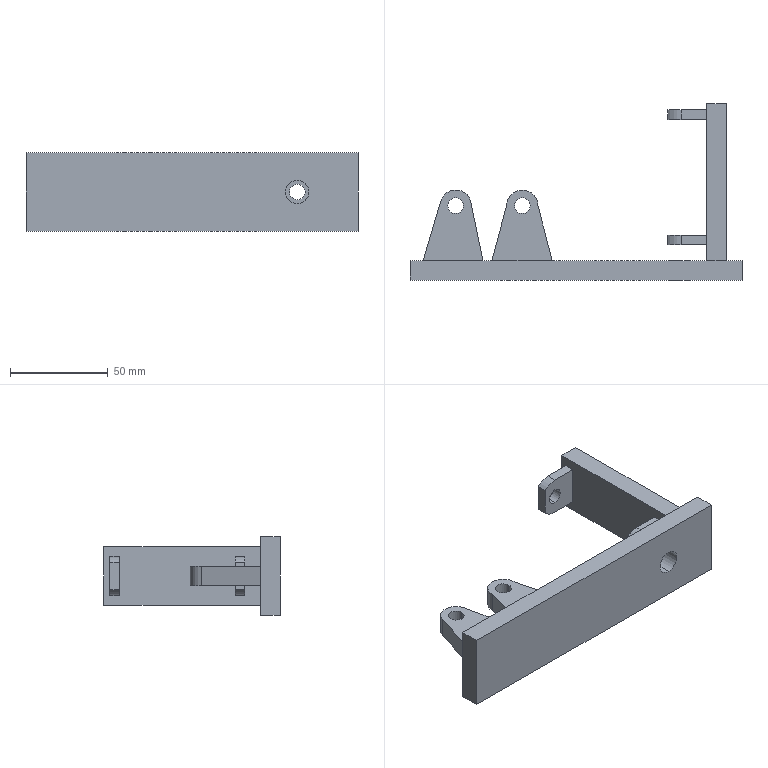Part | SolidWorks | features ICE 5, Extrusion 1 | 1 solid | 45 faces | box 169.404 x 90 x 40 mm | volume 108140 mm3 | plane 29 | cylinder 16 | commonest cylinder face diameters 8 x8 20 x4 12 x2 16 x2
STEP:
#1=CARTESIAN_POINT('',(115.116,-38.,-1.));
#2=VERTEX_POINT('',#1);
#3=CARTESIAN_POINT('',(115.116,-38.,11.));
#4=VERTEX_POINT('',#3);
#5=CARTESIAN_POINT('',(115.116,-38.,5.));
#6=DIRECTION('',(0.,1.,0.));
#7=DIRECTION('',(0.,0.,1.));
#8=AXIS2_PLACEMENT_3D('',#5,#6,#7);
#9=CIRCLE('',#8,6.);
#10=EDGE_CURVE('',#2,#4,#9,.T.);
#11=ORIENTED_EDGE('',*,*,#10,.F.);
#12=CARTESIAN_POINT('',(115.116,-28.,-1.));
#13=VERTEX_POINT('',#12);
#14=CARTESIAN_POINT('',(115.116,-58.,-1.));
#15=DIRECTION('',(0.,1.,0.));
#16=VECTOR('',#15,1000.);
#17=LINE('',#14,#16);
#18=EDGE_CURVE('',#2,#13,#17,.T.);
#19=ORIENTED_EDGE('',*,*,#18,.T.);
#20=CARTESIAN_POINT('',(115.116,-28.,11.));
#21=VERTEX_POINT('',#20);
#22=CARTESIAN_POINT('',(115.116,-28.,5.));
#23=DIRECTION('',(0.,1.,0.));
#24=DIRECTION('',(0.,0.,1.));
#25=AXIS2_PLACEMENT_3D('',#22,#23,#24);
#26=CIRCLE('',#25,6.);
#27=EDGE_CURVE('',#13,#21,#26,.T.);
#28=ORIENTED_EDGE('',*,*,#27,.T.);
#29=CARTESIAN_POINT('',(115.116,-58.,11.));
#30=DIRECTION('',(0.,1.,0.));
#31=VECTOR('',#30,1000.);
#32=LINE('',#29,#31);
#33=EDGE_CURVE('',#4,#21,#32,.T.);
#34=ORIENTED_EDGE('',*,*,#33,.F.);
#35=EDGE_LOOP('',(#11,#19,#28,#34));
#36=FACE_OUTER_BOUND('',#35,.T.);
#37=CARTESIAN_POINT('',(115.116,-58.,5.));
#38=DIRECTION('',(0.,1.,0.));
#39=DIRECTION('',(0.,0.,1.));
#40=AXIS2_PLACEMENT_3D('',#37,#38,#39);
#41=CYLINDRICAL_SURFACE('',#40,6.);
#42=ADVANCED_FACE('',(#36),#41,.F.);
#43=CARTESIAN_POINT('',(115.116,44.,1.));
#44=VERTEX_POINT('',#43);
#45=CARTESIAN_POINT('',(115.116,44.,9.));
#46=VERTEX_POINT('',#45);
#47=CARTESIAN_POINT('',(115.116,44.,5.));
#48=DIRECTION('',(0.,1.,0.));
#49=DIRECTION('',(0.,0.,1.));
#50=AXIS2_PLACEMENT_3D('',#47,#48,#49);
#51=CIRCLE('',#50,4.);
#52=EDGE_CURVE('',#44,#46,#51,.T.);
#53=ORIENTED_EDGE('',*,*,#52,.F.);
#54=CARTESIAN_POINT('',(115.116,49.,1.));
#55=VERTEX_POINT('',#54);
#56=CARTESIAN_POINT('',(115.116,-21.,1.));
#57=DIRECTION('',(0.,1.,0.));
#58=VECTOR('',#57,1000.);
#59=LINE('',#56,#58);
#60=EDGE_CURVE('',#44,#55,#59,.T.);
#61=ORIENTED_EDGE('',*,*,#60,.T.);
#62=CARTESIAN_POINT('',(115.116,49.,9.));
#63=VERTEX_POINT('',#62);
#64=CARTESIAN_POINT('',(115.116,49.,5.));
#65=DIRECTION('',(0.,1.,0.));
#66=DIRECTION('',(0.,0.,1.));
#67=AXIS2_PLACEMENT_3D('',#64,#65,#66);
#68=CIRCLE('',#67,4.);
#69=EDGE_CURVE('',#55,#63,#68,.T.);
#70=ORIENTED_EDGE('',*,*,#69,.T.);
#71=CARTESIAN_POINT('',(115.116,-21.,9.));
#72=DIRECTION('',(0.,1.,0.));
#73=VECTOR('',#72,1000.);
#74=LINE('',#71,#73);
#75=EDGE_CURVE('',#46,#63,#74,.T.);
#76=ORIENTED_EDGE('',*,*,#75,.F.);
#77=EDGE_LOOP('',(#53,#61,#70,#76));
#78=FACE_OUTER_BOUND('',#77,.T.);
#79=CARTESIAN_POINT('',(115.116,-21.,5.));
#80=DIRECTION('',(0.,1.,0.));
#81=DIRECTION('',(0.,0.,1.));
#82=AXIS2_PLACEMENT_3D('',#79,#80,#81);
#83=CYLINDRICAL_SURFACE('',#82,4.);
#84=ADVANCED_FACE('',(#78),#83,.F.);
#85=CARTESIAN_POINT('',(115.116,-20.,1.));
#86=VERTEX_POINT('',#85);
#87=CARTESIAN_POINT('',(115.116,-20.,9.));
#88=VERTEX_POINT('',#87);
#89=CARTESIAN_POINT('',(115.116,-20.,5.));
#90=DIRECTION('',(0.,1.,0.));
#91=DIRECTION('',(0.,0.,1.));
#92=AXIS2_PLACEMENT_3D('',#89,#90,#91);
#93=CIRCLE('',#92,4.);
#94=EDGE_CURVE('',#86,#88,#93,.T.);
#95=ORIENTED_EDGE('',*,*,#94,.F.);
#96=CARTESIAN_POINT('',(115.116,-15.,1.));
#97=VERTEX_POINT('',#96);
#98=CARTESIAN_POINT('',(115.116,-21.,1.));
#99=DIRECTION('',(0.,1.,0.));
#100=VECTOR('',#99,1000.);
#101=LINE('',#98,#100);
#102=EDGE_CURVE('',#86,#97,#101,.T.);
#103=ORIENTED_EDGE('',*,*,#102,.T.);
#104=CARTESIAN_POINT('',(115.116,-15.,9.));
#105=VERTEX_POINT('',#104);
#106=CARTESIAN_POINT('',(115.116,-15.,5.));
#107=DIRECTION('',(0.,-1.,0.));
#108=DIRECTION('',(0.,0.,-1.));
#109=AXIS2_PLACEMENT_3D('',#106,#107,#108);
#110=CIRCLE('',#109,4.);
#111=EDGE_CURVE('',#105,#97,#110,.T.);
#112=ORIENTED_EDGE('',*,*,#111,.F.);
#113=CARTESIAN_POINT('',(115.116,-21.,9.));
#114=DIRECTION('',(0.,1.,0.));
#115=VECTOR('',#114,1000.);
#116=LINE('',#113,#115);
#117=EDGE_CURVE('',#88,#105,#116,.T.);
#118=ORIENTED_EDGE('',*,*,#117,.F.);
#119=EDGE_LOOP('',(#95,#103,#112,#118));
#120=FACE_OUTER_BOUND('',#119,.T.);
#121=CARTESIAN_POINT('',(115.116,-21.,5.));
#122=DIRECTION('',(0.,1.,0.));
#123=DIRECTION('',(0.,0.,1.));
#124=AXIS2_PLACEMENT_3D('',#121,#122,#123);
#125=CYLINDRICAL_SURFACE('',#124,4.);
#126=ADVANCED_FACE('',(#120),#125,.F.);
#127=CARTESIAN_POINT('',(30.,0.,10.));
#128=VERTEX_POINT('',#127);
#129=CARTESIAN_POINT('',(38.,0.,10.));
#130=VERTEX_POINT('',#129);
#131=CARTESIAN_POINT('',(34.,0.,10.));
#132=DIRECTION('',(0.,0.,1.));
#133=DIRECTION('',(1.,0.,0.));
#134=AXIS2_PLACEMENT_3D('',#131,#132,#133);
#135=CIRCLE('',#134,4.);
#136=EDGE_CURVE('',#128,#130,#135,.T.);
#137=ORIENTED_EDGE('',*,*,#136,.T.);
#138=CARTESIAN_POINT('',(38.,0.,0.));
#139=VERTEX_POINT('',#138);
#140=CARTESIAN_POINT('',(38.,0.,10.));
#141=DIRECTION('',(0.,0.,-1.));
#142=VECTOR('',#141,1000.);
#143=LINE('',#140,#142);
#144=EDGE_CURVE('',#130,#139,#143,.T.);
#145=ORIENTED_EDGE('',*,*,#144,.T.);
#146=CARTESIAN_POINT('',(30.,0.,0.));
#147=VERTEX_POINT('',#146);
#148=CARTESIAN_POINT('',(34.,0.,0.));
#149=DIRECTION('',(0.,0.,1.));
#150=DIRECTION('',(1.,0.,0.));
#151=AXIS2_PLACEMENT_3D('',#148,#149,#150);
#152=CIRCLE('',#151,4.);
#153=EDGE_CURVE('',#147,#139,#152,.T.);
#154=ORIENTED_EDGE('',*,*,#153,.F.);
#155=CARTESIAN_POINT('',(30.,0.,10.));
#156=DIRECTION('',(0.,0.,-1.));
#157=VECTOR('',#156,1000.);
#158=LINE('',#155,#157);
#159=EDGE_CURVE('',#128,#147,#158,.T.);
#160=ORIENTED_EDGE('',*,*,#159,.F.);
#161=EDGE_LOOP('',(#137,#145,#154,#160));
#162=FACE_OUTER_BOUND('',#161,.T.);
#163=CARTESIAN_POINT('',(34.,0.,10.));
#164=DIRECTION('',(0.,0.,-1.));
#165=DIRECTION('',(-1.,0.,0.));
#166=AXIS2_PLACEMENT_3D('',#163,#164,#165);
#167=CYLINDRICAL_SURFACE('',#166,4.);
#168=ADVANCED_FACE('',(#162),#167,.F.);
#169=CARTESIAN_POINT('',(-4.,0.,10.));
#170=VERTEX_POINT('',#169);
#171=CARTESIAN_POINT('',(4.,0.,10.));
#172=VERTEX_POINT('',#171);
#173=CARTESIAN_POINT('',(0.,0.,10.));
#174=DIRECTION('',(0.,0.,1.));
#175=DIRECTION('',(1.,0.,0.));
#176=AXIS2_PLACEMENT_3D('',#173,#174,#175);
#177=CIRCLE('',#176,4.);
#178=EDGE_CURVE('',#170,#172,#177,.T.);
#179=ORIENTED_EDGE('',*,*,#178,.T.);
#180=CARTESIAN_POINT('',(4.,0.,0.));
#181=VERTEX_POINT('',#180);
#182=CARTESIAN_POINT('',(4.,0.,10.));
#183=DIRECTION('',(0.,0.,-1.));
#184=VECTOR('',#183,1000.);
#185=LINE('',#182,#184);
#186=EDGE_CURVE('',#172,#181,#185,.T.);
#187=ORIENTED_EDGE('',*,*,#186,.T.);
#188=CARTESIAN_POINT('',(-4.,0.,0.));
#189=VERTEX_POINT('',#188);
#190=CARTESIAN_POINT('',(0.,0.,0.));
#191=DIRECTION('',(0.,0.,1.));
#192=DIRECTION('',(1.,0.,0.));
#193=AXIS2_PLACEMENT_3D('',#190,#191,#192);
#194=CIRCLE('',#193,4.);
#195=EDGE_CURVE('',#189,#181,#194,.T.);
#196=ORIENTED_EDGE('',*,*,#195,.F.);
#197=CARTESIAN_POINT('',(-4.,0.,10.));
#198=DIRECTION('',(0.,0.,-1.));
#199=VECTOR('',#198,1000.);
#200=LINE('',#197,#199);
#201=EDGE_CURVE('',#170,#189,#200,.T.);
#202=ORIENTED_EDGE('',*,*,#201,.F.);
#203=EDGE_LOOP('',(#179,#187,#196,#202));
#204=FACE_OUTER_BOUND('',#203,.T.);
#205=CARTESIAN_POINT('',(0.,0.,10.));
#206=DIRECTION('',(0.,0.,-1.));
#207=DIRECTION('',(-1.,0.,0.));
#208=AXIS2_PLACEMENT_3D('',#205,#206,#207);
#209=CYLINDRICAL_SURFACE('',#208,4.);
#210=ADVANCED_FACE('',(#204),#209,.F.);
#211=CARTESIAN_POINT('',(115.116,44.,-5.));
#212=VERTEX_POINT('',#211);
#213=CARTESIAN_POINT('',(115.116,49.,-5.));
#214=VERTEX_POINT('',#213);
#215=CARTESIAN_POINT('',(115.116,-21.,-5.));
#216=DIRECTION('',(0.,1.,0.));
#217=VECTOR('',#216,1000.);
#218=LINE('',#215,#217);
#219=EDGE_CURVE('',#212,#214,#218,.T.);
#220=ORIENTED_EDGE('',*,*,#219,.T.);
#221=CARTESIAN_POINT('',(128.116,49.,-5.));
#222=VERTEX_POINT('',#221);
#223=CARTESIAN_POINT('',(108.116,49.,-5.));
#224=DIRECTION('',(1.,0.,0.));
#225=VECTOR('',#224,1000.);
#226=LINE('',#223,#225);
#227=EDGE_CURVE('',#214,#222,#226,.T.);
#228=ORIENTED_EDGE('',*,*,#227,.T.);
#229=CARTESIAN_POINT('',(128.116,44.,-5.));
#230=VERTEX_POINT('',#229);
#231=CARTESIAN_POINT('',(128.116,49.,-5.));
#232=DIRECTION('',(0.,-1.,0.));
#233=VECTOR('',#232,1000.);
#234=LINE('',#231,#233);
#235=EDGE_CURVE('',#222,#230,#234,.T.);
#236=ORIENTED_EDGE('',*,*,#235,.T.);
#237=CARTESIAN_POINT('',(108.116,44.,-5.));
#238=DIRECTION('',(1.,0.,0.));
#239=VECTOR('',#238,1000.);
#240=LINE('',#237,#239);
#241=EDGE_CURVE('',#212,#230,#240,.T.);
#242=ORIENTED_EDGE('',*,*,#241,.F.);
#243=EDGE_LOOP('',(#220,#228,#236,#242));
#244=FACE_OUTER_BOUND('',#243,.T.);
#245=CARTESIAN_POINT('',(108.116,49.,-5.));
#246=DIRECTION('',(0.,0.,1.));
#247=DIRECTION('',(0.,-1.,0.));
#248=AXIS2_PLACEMENT_3D('',#245,#246,#247);
#249=PLANE('',#248);
#250=ADVANCED_FACE('',(#244),#249,.F.);
#251=CARTESIAN_POINT('',(115.116,-20.,-5.));
#252=VERTEX_POINT('',#251);
#253=CARTESIAN_POINT('',(115.116,-15.,-5.));
#254=VERTEX_POINT('',#253);
#255=CARTESIAN_POINT('',(115.116,-21.,-5.));
#256=DIRECTION('',(0.,1.,0.));
#257=VECTOR('',#256,1000.);
#258=LINE('',#255,#257);
#259=EDGE_CURVE('',#252,#254,#258,.T.);
#260=ORIENTED_EDGE('',*,*,#259,.T.);
#261=CARTESIAN_POINT('',(128.116,-15.,-5.));
#262=VERTEX_POINT('',#261);
#263=CARTESIAN_POINT('',(108.116,-15.,-5.));
#264=DIRECTION('',(1.,0.,0.));
#265=VECTOR('',#264,1000.);
#266=LINE('',#263,#265);
#267=EDGE_CURVE('',#254,#262,#266,.T.);
#268=ORIENTED_EDGE('',*,*,#267,.T.);
#269=CARTESIAN_POINT('',(128.116,-20.,-5.));
#270=VERTEX_POINT('',#269);
#271=CARTESIAN_POINT('',(128.116,-15.,-5.));
#272=DIRECTION('',(0.,-1.,0.));
#273=VECTOR('',#272,1000.);
#274=LINE('',#271,#273);
#275=EDGE_CURVE('',#262,#270,#274,.T.);
#276=ORIENTED_EDGE('',*,*,#275,.T.);
#277=CARTESIAN_POINT('',(108.116,-20.,-5.));
#278=DIRECTION('',(1.,0.,0.));
#279=VECTOR('',#278,1000.);
#280=LINE('',#277,#279);
#281=EDGE_CURVE('',#252,#270,#280,.T.);
#282=ORIENTED_EDGE('',*,*,#281,.F.);
#283=EDGE_LOOP('',(#260,#268,#276,#282));
#284=FACE_OUTER_BOUND('',#283,.T.);
#285=CARTESIAN_POINT('',(108.116,-15.,-5.));
#286=DIRECTION('',(0.,0.,1.));
#287=DIRECTION('',(0.,-1.,0.));
#288=AXIS2_PLACEMENT_3D('',#285,#286,#287);
#289=PLANE('',#288);
#290=ADVANCED_FACE('',(#284),#289,.F.);
#291=CARTESIAN_POINT('',(128.116,44.,15.));
#292=VERTEX_POINT('',#291);
#293=CARTESIAN_POINT('',(128.116,49.,15.));
#294=VERTEX_POINT('',#293);
#295=CARTESIAN_POINT('',(128.116,49.,15.));
#296=DIRECTION('',(0.,1.,0.));
#297=VECTOR('',#296,1000.);
#298=LINE('',#295,#297);
#299=EDGE_CURVE('',#292,#294,#298,.T.);
#300=ORIENTED_EDGE('',*,*,#299,.F.);
#301=CARTESIAN_POINT('',(128.116,44.,-5.));
#302=DIRECTION('',(0.,0.,1.));
#303=VECTOR('',#302,1000.);
#304=LINE('',#301,#303);
#305=EDGE_CURVE('',#230,#292,#304,.T.);
#306=ORIENTED_EDGE('',*,*,#305,.F.);
#307=ORIENTED_EDGE('',*,*,#235,.F.);
#308=CARTESIAN_POINT('',(128.116,49.,-5.));
#309=DIRECTION('',(0.,0.,-1.));
#310=VECTOR('',#309,1000.);
#311=LINE('',#308,#310);
#312=EDGE_CURVE('',#294,#222,#311,.T.);
#313=ORIENTED_EDGE('',*,*,#312,.F.);
#314=EDGE_LOOP('',(#300,#306,#307,#313));
#315=FACE_BOUND('',#314,.T.);
#316=CARTESIAN_POINT('',(128.116,-28.,-10.));
#317=VERTEX_POINT('',#316);
#318=CARTESIAN_POINT('',(128.116,-28.,20.));
#319=VERTEX_POINT('',#318);
#320=CARTESIAN_POINT('',(128.116,-28.,-10.));
#321=DIRECTION('',(0.,0.,1.));
#322=VECTOR('',#321,1000.);
#323=LINE('',#320,#322);
#324=EDGE_CURVE('',#317,#319,#323,.T.);
#325=ORIENTED_EDGE('',*,*,#324,.T.);
#326=CARTESIAN_POINT('',(128.116,52.,20.));
#327=VERTEX_POINT('',#326);
#328=CARTESIAN_POINT('',(128.116,52.,20.));
#329=DIRECTION('',(0.,-1.,0.));
#330=VECTOR('',#329,1000.);
#331=LINE('',#328,#330);
#332=EDGE_CURVE('',#327,#319,#331,.T.);
#333=ORIENTED_EDGE('',*,*,#332,.F.);
#334=CARTESIAN_POINT('',(128.116,52.,-10.));
#335=VERTEX_POINT('',#334);
#336=CARTESIAN_POINT('',(128.116,52.,-10.));
#337=DIRECTION('',(0.,0.,1.));
#338=VECTOR('',#337,1000.);
#339=LINE('',#336,#338);
#340=EDGE_CURVE('',#335,#327,#339,.T.);
#341=ORIENTED_EDGE('',*,*,#340,.F.);
#342=CARTESIAN_POINT('',(128.116,52.,-10.));
#343=DIRECTION('',(0.,-1.,0.));
#344=VECTOR('',#343,1000.);
#345=LINE('',#342,#344);
#346=EDGE_CURVE('',#335,#317,#345,.T.);
#347=ORIENTED_EDGE('',*,*,#346,.T.);
#348=EDGE_LOOP('',(#325,#333,#341,#347));
#349=FACE_OUTER_BOUND('',#348,.T.);
#350=CARTESIAN_POINT('',(128.116,-20.,15.));
#351=VERTEX_POINT('',#350);
#352=CARTESIAN_POINT('',(128.116,-15.,15.));
#353=VERTEX_POINT('',#352);
#354=CARTESIAN_POINT('',(128.116,-15.,15.));
#355=DIRECTION('',(0.,1.,0.));
#356=VECTOR('',#355,1000.);
#357=LINE('',#354,#356);
#358=EDGE_CURVE('',#351,#353,#357,.T.);
#359=ORIENTED_EDGE('',*,*,#358,.F.);
#360=CARTESIAN_POINT('',(128.116,-20.,-5.));
#361=DIRECTION('',(0.,0.,1.));
#362=VECTOR('',#361,1000.);
#363=LINE('',#360,#362);
#364=EDGE_CURVE('',#270,#351,#363,.T.);
#365=ORIENTED_EDGE('',*,*,#364,.F.);
#366=ORIENTED_EDGE('',*,*,#275,.F.);
#367=CARTESIAN_POINT('',(128.116,-15.,-5.));
#368=DIRECTION('',(0.,0.,-1.));
#369=VECTOR('',#368,1000.);
#370=LINE('',#367,#369);
#371=EDGE_CURVE('',#353,#262,#370,.T.);
#372=ORIENTED_EDGE('',*,*,#371,.F.);
#373=EDGE_LOOP('',(#359,#365,#366,#372));
#374=FACE_BOUND('',#373,.T.);
#375=CARTESIAN_POINT('',(128.116,52.,-10.));
#376=DIRECTION('',(1.,0.,0.));
#377=DIRECTION('',(0.,0.,-1.));
#378=AXIS2_PLACEMENT_3D('',#375,#376,#377);
#379=PLANE('',#378);
#380=ADVANCED_FACE('',(#315,#349,#374),#379,.F.);
#381=CARTESIAN_POINT('',(115.116,-28.,5.));
#382=DIRECTION('',(0.,1.,0.));
#383=DIRECTION('',(0.,0.,1.));
#384=AXIS2_PLACEMENT_3D('',#381,#382,#383);
#385=CIRCLE('',#384,6.);
#386=EDGE_CURVE('',#21,#13,#385,.T.);
#387=ORIENTED_EDGE('',*,*,#386,.F.);
#388=ORIENTED_EDGE('',*,*,#27,.F.);
#389=EDGE_LOOP('',(#387,#388));
#390=FACE_BOUND('',#389,.T.);
#391=CARTESIAN_POINT('',(-23.288,-28.,25.));
#392=VERTEX_POINT('',#391);
#393=CARTESIAN_POINT('',(-23.288,-28.,-15.));
#394=VERTEX_POINT('',#393);
#395=CARTESIAN_POINT('',(-23.288,-28.,-15.));
#396=DIRECTION('',(0.,0.,-1.));
#397=VECTOR('',#396,1000.);
#398=LINE('',#395,#397);
#399=EDGE_CURVE('',#392,#394,#398,.T.);
#400=ORIENTED_EDGE('',*,*,#399,.F.);
#401=CARTESIAN_POINT('',(146.116,-28.,25.));
#402=VERTEX_POINT('',#401);
#403=CARTESIAN_POINT('',(146.116,-28.,25.));
#404=DIRECTION('',(-1.,0.,0.));
#405=VECTOR('',#404,1000.);
#406=LINE('',#403,#405);
#407=EDGE_CURVE('',#402,#392,#406,.T.);
#408=ORIENTED_EDGE('',*,*,#407,.F.);
#409=CARTESIAN_POINT('',(146.116,-28.,-15.));
#410=VERTEX_POINT('',#409);
#411=CARTESIAN_POINT('',(146.116,-28.,-15.));
#412=DIRECTION('',(0.,0.,1.));
#413=VECTOR('',#412,1000.);
#414=LINE('',#411,#413);
#415=EDGE_CURVE('',#410,#402,#414,.T.);
#416=ORIENTED_EDGE('',*,*,#415,.F.);
#417=CARTESIAN_POINT('',(146.116,-28.,-15.));
#418=DIRECTION('',(1.,0.,0.));
#419=VECTOR('',#418,1000.);
#420=LINE('',#417,#419);
#421=EDGE_CURVE('',#394,#410,#420,.T.);
#422=ORIENTED_EDGE('',*,*,#421,.F.);
#423=EDGE_LOOP('',(#400,#408,#416,#422));
#424=FACE_OUTER_BOUND('',#423,.T.);
#425=CARTESIAN_POINT('',(18.477,-28.,10.));
#426=VERTEX_POINT('',#425);
#427=CARTESIAN_POINT('',(18.477,-28.,0.));
#428=VERTEX_POINT('',#427);
#429=CARTESIAN_POINT('',(18.477,-28.,10.));
#430=DIRECTION('',(0.,0.,-1.));
#431=VECTOR('',#430,1000.);
#432=LINE('',#429,#431);
#433=EDGE_CURVE('',#426,#428,#432,.T.);
#434=ORIENTED_EDGE('',*,*,#433,.T.);
#435=CARTESIAN_POINT('',(49.273,-28.,0.));
#436=VERTEX_POINT('',#435);
#437=CARTESIAN_POINT('',(0.,-28.,0.));
#438=DIRECTION('',(1.,0.,0.));
#439=VECTOR('',#438,1000.);
#440=LINE('',#437,#439);
#441=EDGE_CURVE('',#428,#436,#440,.T.);
#442=ORIENTED_EDGE('',*,*,#441,.T.);
#443=CARTESIAN_POINT('',(49.273,-28.,10.));
#444=VERTEX_POINT('',#443);
#445=CARTESIAN_POINT('',(49.273,-28.,10.));
#446=DIRECTION('',(0.,0.,1.));
#447=VECTOR('',#446,1000.);
#448=LINE('',#445,#447);
#449=EDGE_CURVE('',#436,#444,#448,.T.);
#450=ORIENTED_EDGE('',*,*,#449,.T.);
#451=CARTESIAN_POINT('',(0.,-28.,10.));
#452=DIRECTION('',(1.,0.,0.));
#453=VECTOR('',#452,1000.);
#454=LINE('',#451,#453);
#455=EDGE_CURVE('',#426,#444,#454,.T.);
#456=ORIENTED_EDGE('',*,*,#455,.F.);
#457=EDGE_LOOP('',(#434,#442,#450,#456));
#458=FACE_BOUND('',#457,.T.);
#459=CARTESIAN_POINT('',(13.917,-28.,10.));
#460=VERTEX_POINT('',#459);
#461=CARTESIAN_POINT('',(13.917,-28.,0.));
#462=VERTEX_POINT('',#461);
#463=CARTESIAN_POINT('',(13.917,-28.,10.));
#464=DIRECTION('',(0.,0.,-1.));
#465=VECTOR('',#464,1000.);
#466=LINE('',#463,#465);
#467=EDGE_CURVE('',#460,#462,#466,.T.);
#468=ORIENTED_EDGE('',*,*,#467,.F.);
#469=CARTESIAN_POINT('',(-16.58,-28.,10.));
#470=VERTEX_POINT('',#469);
#471=CARTESIAN_POINT('',(0.,-28.,10.));
#472=DIRECTION('',(1.,0.,0.));
#473=VECTOR('',#472,1000.);
#474=LINE('',#471,#473);
#475=EDGE_CURVE('',#470,#460,#474,.T.);
#476=ORIENTED_EDGE('',*,*,#475,.F.);
#477=CARTESIAN_POINT('',(-16.58,-28.,0.));
#478=VERTEX_POINT('',#477);
#479=CARTESIAN_POINT('',(-16.58,-28.,10.));
#480=DIRECTION('',(0.,0.,-1.));
#481=VECTOR('',#480,1000.);
#482=LINE('',#479,#481);
#483=EDGE_CURVE('',#470,#478,#482,.T.);
#484=ORIENTED_EDGE('',*,*,#483,.T.);
#485=CARTESIAN_POINT('',(0.,-28.,0.));
#486=DIRECTION('',(1.,0.,0.));
#487=VECTOR('',#486,1000.);
#488=LINE('',#485,#487);
#489=EDGE_CURVE('',#478,#462,#488,.T.);
#490=ORIENTED_EDGE('',*,*,#489,.T.);
#491=EDGE_LOOP('',(#468,#476,#484,#490));
#492=FACE_BOUND('',#491,.T.);
#493=CARTESIAN_POINT('',(138.116,-28.,20.));
#494=VERTEX_POINT('',#493);
#495=CARTESIAN_POINT('',(138.116,-28.,-10.));
#496=VERTEX_POINT('',#495);
#497=CARTESIAN_POINT('',(138.116,-28.,-10.));
#498=DIRECTION('',(0.,0.,-1.));
#499=VECTOR('',#498,1000.);
#500=LINE('',#497,#499);
#501=EDGE_CURVE('',#494,#496,#500,.T.);
#502=ORIENTED_EDGE('',*,*,#501,.F.);
#503=CARTESIAN_POINT('',(128.116,-28.,20.));
#504=DIRECTION('',(1.,0.,0.));
#505=VECTOR('',#504,1000.);
#506=LINE('',#503,#505);
#507=EDGE_CURVE('',#319,#494,#506,.T.);
#508=ORIENTED_EDGE('',*,*,#507,.F.);
#509=ORIENTED_EDGE('',*,*,#324,.F.);
#510=CARTESIAN_POINT('',(128.116,-28.,-10.));
#511=DIRECTION('',(-1.,0.,0.));
#512=VECTOR('',#511,1000.);
#513=LINE('',#510,#512);
#514=EDGE_CURVE('',#496,#317,#513,.T.);
#515=ORIENTED_EDGE('',*,*,#514,.F.);
#516=EDGE_LOOP('',(#502,#508,#509,#515));
#517=FACE_BOUND('',#516,.T.);
#518=CARTESIAN_POINT('',(13.917,-28.,10.));
#519=DIRECTION('',(0.,-1.,0.));
#520=DIRECTION('',(0.,0.,-1.));
#521=AXIS2_PLACEMENT_3D('',#518,#519,#520);
#522=PLANE('',#521);
#523=ADVANCED_FACE('',(#390,#424,#458,#492,#517),#522,.F.);
#524=ORIENTED_EDGE('',*,*,#178,.F.);
#525=CARTESIAN_POINT('',(0.,0.,10.));
#526=DIRECTION('',(0.,0.,1.));
#527=DIRECTION('',(1.,0.,0.));
#528=AXIS2_PLACEMENT_3D('',#525,#526,#527);
#529=CIRCLE('',#528,4.);
#530=EDGE_CURVE('',#172,#170,#529,.T.);
#531=ORIENTED_EDGE('',*,*,#530,.F.);
#532=EDGE_LOOP('',(#524,#531));
#533=FACE_BOUND('',#532,.T.);
#534=CARTESIAN_POINT('',(-7.675,2.259,10.));
#535=VERTEX_POINT('',#534);
#536=CARTESIAN_POINT('',(-7.675,2.259,10.));
#537=DIRECTION('',(-0.2823,-0.9593,0.));
#538=VECTOR('',#537,1000.);
#539=LINE('',#536,#538);
#540=EDGE_CURVE('',#535,#470,#539,.T.);
#541=ORIENTED_EDGE('',*,*,#540,.T.);
#542=ORIENTED_EDGE('',*,*,#475,.T.);
#543=CARTESIAN_POINT('',(7.675,2.259,10.));
#544=VERTEX_POINT('',#543);
#545=CARTESIAN_POINT('',(7.675,2.259,10.));
#546=DIRECTION('',(-0.202,0.9794,0.));
#547=VECTOR('',#546,1000.);
#548=LINE('',#545,#547);
#549=EDGE_CURVE('',#460,#544,#548,.T.);
#550=ORIENTED_EDGE('',*,*,#549,.T.);
#551=CARTESIAN_POINT('',(0.,0.,10.));
#552=DIRECTION('',(0.,0.,1.));
#553=DIRECTION('',(1.,0.,0.));
#554=AXIS2_PLACEMENT_3D('',#551,#552,#553);
#555=CIRCLE('',#554,8.);
#556=EDGE_CURVE('',#544,#535,#555,.T.);
#557=ORIENTED_EDGE('',*,*,#556,.T.);
#558=EDGE_LOOP('',(#541,#542,#550,#557));
#559=FACE_OUTER_BOUND('',#558,.T.);
#560=CARTESIAN_POINT('',(0.,0.,10.));
#561=DIRECTION('',(0.,0.,1.));
#562=DIRECTION('',(1.,0.,0.));
#563=AXIS2_PLACEMENT_3D('',#560,#561,#562);
#564=PLANE('',#563);
#565=ADVANCED_FACE('',(#533,#559),#564,.T.);
#566=ORIENTED_EDGE('',*,*,#136,.F.);
#567=CARTESIAN_POINT('',(34.,0.,10.));
#568=DIRECTION('',(0.,0.,1.));
#569=DIRECTION('',(1.,0.,0.));
#570=AXIS2_PLACEMENT_3D('',#567,#568,#569);
#571=CIRCLE('',#570,4.);
#572=EDGE_CURVE('',#130,#128,#571,.T.);
#573=ORIENTED_EDGE('',*,*,#572,.F.);
#574=EDGE_LOOP('',(#566,#573));
#575=FACE_BOUND('',#574,.T.);
#576=CARTESIAN_POINT('',(26.,0.,10.));
#577=VERTEX_POINT('',#576);
#578=CARTESIAN_POINT('',(26.,0.,10.));
#579=DIRECTION('',(-0.2595,-0.9657,0.));
#580=VECTOR('',#579,1000.);
#581=LINE('',#578,#580);
#582=EDGE_CURVE('',#577,#426,#581,.T.);
#583=ORIENTED_EDGE('',*,*,#582,.T.);
#584=ORIENTED_EDGE('',*,*,#455,.T.);
#585=CARTESIAN_POINT('',(42.,0.,10.));
#586=VERTEX_POINT('',#585);
#587=CARTESIAN_POINT('',(49.355,-28.317,10.));
#588=DIRECTION('',(-0.2514,0.9679,0.));
#589=VECTOR('',#588,1000.);
#590=LINE('',#587,#589);
#591=EDGE_CURVE('',#444,#586,#590,.T.);
#592=ORIENTED_EDGE('',*,*,#591,.T.);
#593=CARTESIAN_POINT('',(34.,0.,10.));
#594=DIRECTION('',(0.,0.,1.));
#595=DIRECTION('',(1.,0.,0.));
#596=AXIS2_PLACEMENT_3D('',#593,#594,#595);
#597=CIRCLE('',#596,8.);
#598=EDGE_CURVE('',#586,#577,#597,.T.);
#599=ORIENTED_EDGE('',*,*,#598,.T.);
#600=EDGE_LOOP('',(#583,#584,#592,#599));
#601=FACE_OUTER_BOUND('',#600,.T.);
#602=CARTESIAN_POINT('',(0.,0.,10.));
#603=DIRECTION('',(0.,0.,1.));
#604=DIRECTION('',(1.,0.,0.));
#605=AXIS2_PLACEMENT_3D('',#602,#603,#604);
#606=PLANE('',#605);
#607=ADVANCED_FACE('',(#575,#601),#606,.T.);
#608=ORIENTED_EDGE('',*,*,#195,.T.);
#609=CARTESIAN_POINT('',(0.,0.,0.));
#610=DIRECTION('',(0.,0.,1.));
#611=DIRECTION('',(1.,0.,0.));
#612=AXIS2_PLACEMENT_3D('',#609,#610,#611);
#613=CIRCLE('',#612,4.);
#614=EDGE_CURVE('',#181,#189,#613,.T.);
#615=ORIENTED_EDGE('',*,*,#614,.T.);
#616=EDGE_LOOP('',(#608,#615));
#617=FACE_BOUND('',#616,.T.);
#618=ORIENTED_EDGE('',*,*,#489,.F.);
#619=CARTESIAN_POINT('',(-7.675,2.259,0.));
#620=VERTEX_POINT('',#619);
#621=CARTESIAN_POINT('',(-7.675,2.259,0.));
#622=DIRECTION('',(-0.2823,-0.9593,0.));
#623=VECTOR('',#622,1000.);
#624=LINE('',#621,#623);
#625=EDGE_CURVE('',#620,#478,#624,.T.);
#626=ORIENTED_EDGE('',*,*,#625,.F.);
#627=CARTESIAN_POINT('',(7.675,2.259,0.));
#628=VERTEX_POINT('',#627);
#629=CARTESIAN_POINT('',(0.,0.,0.));
#630=DIRECTION('',(0.,0.,1.));
#631=DIRECTION('',(1.,0.,0.));
#632=AXIS2_PLACEMENT_3D('',#629,#630,#631);
#633=CIRCLE('',#632,8.);
#634=EDGE_CURVE('',#628,#620,#633,.T.);
#635=ORIENTED_EDGE('',*,*,#634,.F.);
#636=CARTESIAN_POINT('',(7.675,2.259,0.));
#637=DIRECTION('',(-0.202,0.9794,0.));
#638=VECTOR('',#637,1000.);
#639=LINE('',#636,#638);
#640=EDGE_CURVE('',#462,#628,#639,.T.);
#641=ORIENTED_EDGE('',*,*,#640,.F.);
#642=EDGE_LOOP('',(#618,#626,#635,#641));
#643=FACE_OUTER_BOUND('',#642,.T.);
#644=CARTESIAN_POINT('',(0.,0.,0.));
#645=DIRECTION('',(0.,0.,1.));
#646=DIRECTION('',(1.,0.,0.));
#647=AXIS2_PLACEMENT_3D('',#644,#645,#646);
#648=PLANE('',#647);
#649=ADVANCED_FACE('',(#617,#643),#648,.F.);
#650=ORIENTED_EDGE('',*,*,#153,.T.);
#651=CARTESIAN_POINT('',(34.,0.,0.));
#652=DIRECTION('',(0.,0.,1.));
#653=DIRECTION('',(1.,0.,0.));
#654=AXIS2_PLACEMENT_3D('',#651,#652,#653);
#655=CIRCLE('',#654,4.);
#656=EDGE_CURVE('',#139,#147,#655,.T.);
#657=ORIENTED_EDGE('',*,*,#656,.T.);
#658=EDGE_LOOP('',(#650,#657));
#659=FACE_BOUND('',#658,.T.);
#660=ORIENTED_EDGE('',*,*,#441,.F.);
#661=CARTESIAN_POINT('',(26.,0.,0.));
#662=VERTEX_POINT('',#661);
#663=CARTESIAN_POINT('',(26.,0.,0.));
#664=DIRECTION('',(-0.2595,-0.9657,0.));
#665=VECTOR('',#664,1000.);
#666=LINE('',#663,#665);
#667=EDGE_CURVE('',#662,#428,#666,.T.);
#668=ORIENTED_EDGE('',*,*,#667,.F.);
#669=CARTESIAN_POINT('',(42.,0.,0.));
#670=VERTEX_POINT('',#669);
#671=CARTESIAN_POINT('',(34.,0.,0.));
#672=DIRECTION('',(0.,0.,1.));
#673=DIRECTION('',(1.,0.,0.));
#674=AXIS2_PLACEMENT_3D('',#671,#672,#673);
#675=CIRCLE('',#674,8.);
#676=EDGE_CURVE('',#670,#662,#675,.T.);
#677=ORIENTED_EDGE('',*,*,#676,.F.);
#678=CARTESIAN_POINT('',(49.355,-28.317,0.));
#679=DIRECTION('',(-0.2514,0.9679,0.));
#680=VECTOR('',#679,1000.);
#681=LINE('',#678,#680);
#682=EDGE_CURVE('',#436,#670,#681,.T.);
#683=ORIENTED_EDGE('',*,*,#682,.F.);
#684=EDGE_LOOP('',(#660,#668,#677,#683));
#685=FACE_OUTER_BOUND('',#684,.T.);
#686=CARTESIAN_POINT('',(0.,0.,0.));
#687=DIRECTION('',(0.,0.,1.));
#688=DIRECTION('',(1.,0.,0.));
#689=AXIS2_PLACEMENT_3D('',#686,#687,#688);
#690=PLANE('',#689);
#691=ADVANCED_FACE('',(#659,#685),#690,.F.);
#692=ORIENTED_EDGE('',*,*,#449,.F.);
#693=ORIENTED_EDGE('',*,*,#682,.T.);
#694=CARTESIAN_POINT('',(42.,0.,10.));
#695=DIRECTION('',(0.,0.,-1.));
#696=VECTOR('',#695,1000.);
#697=LINE('',#694,#696);
#698=EDGE_CURVE('',#586,#670,#697,.T.);
#699=ORIENTED_EDGE('',*,*,#698,.F.);
#700=ORIENTED_EDGE('',*,*,#591,.F.);
#701=EDGE_LOOP('',(#692,#693,#699,#700));
#702=FACE_OUTER_BOUND('',#701,.T.);
#703=CARTESIAN_POINT('',(49.355,-28.317,10.));
#704=DIRECTION('',(-0.9679,-0.2514,0.));
#705=DIRECTION('',(0.2514,-0.9679,0.));
#706=AXIS2_PLACEMENT_3D('',#703,#704,#705);
#707=PLANE('',#706);
#708=ADVANCED_FACE('',(#702),#707,.F.);
#709=ORIENTED_EDGE('',*,*,#634,.T.);
#710=CARTESIAN_POINT('',(-7.675,2.259,10.));
#711=DIRECTION('',(0.,0.,-1.));
#712=VECTOR('',#711,1000.);
#713=LINE('',#710,#712);
#714=EDGE_CURVE('',#535,#620,#713,.T.);
#715=ORIENTED_EDGE('',*,*,#714,.F.);
#716=ORIENTED_EDGE('',*,*,#556,.F.);
#717=CARTESIAN_POINT('',(7.675,2.259,10.));
#718=DIRECTION('',(0.,0.,-1.));
#719=VECTOR('',#718,1000.);
#720=LINE('',#717,#719);
#721=EDGE_CURVE('',#544,#628,#720,.T.);
#722=ORIENTED_EDGE('',*,*,#721,.T.);
#723=EDGE_LOOP('',(#709,#715,#716,#722));
#724=FACE_OUTER_BOUND('',#723,.T.);
#725=CARTESIAN_POINT('',(0.,0.,10.));
#726=DIRECTION('',(0.,0.,-1.));
#727=DIRECTION('',(-1.,0.,0.));
#728=AXIS2_PLACEMENT_3D('',#725,#726,#727);
#729=CYLINDRICAL_SURFACE('',#728,8.);
#730=ADVANCED_FACE('',(#724),#729,.T.);
#731=ORIENTED_EDGE('',*,*,#625,.T.);
#732=ORIENTED_EDGE('',*,*,#483,.F.);
#733=ORIENTED_EDGE('',*,*,#540,.F.);
#734=ORIENTED_EDGE('',*,*,#714,.T.);
#735=EDGE_LOOP('',(#731,#732,#733,#734));
#736=FACE_OUTER_BOUND('',#735,.T.);
#737=CARTESIAN_POINT('',(-7.675,2.259,10.));
#738=DIRECTION('',(0.9593,-0.2823,0.));
#739=DIRECTION('',(0.2823,0.9593,0.));
#740=AXIS2_PLACEMENT_3D('',#737,#738,#739);
#741=PLANE('',#740);
#742=ADVANCED_FACE('',(#736),#741,.F.);
#743=ORIENTED_EDGE('',*,*,#676,.T.);
#744=CARTESIAN_POINT('',(26.,0.,10.));
#745=DIRECTION('',(0.,0.,-1.));
#746=VECTOR('',#745,1000.);
#747=LINE('',#744,#746);
#748=EDGE_CURVE('',#577,#662,#747,.T.);
#749=ORIENTED_EDGE('',*,*,#748,.F.);
#750=ORIENTED_EDGE('',*,*,#598,.F.);
#751=ORIENTED_EDGE('',*,*,#698,.T.);
#752=EDGE_LOOP('',(#743,#749,#750,#751));
#753=FACE_OUTER_BOUND('',#752,.T.);
#754=CARTESIAN_POINT('',(34.,0.,10.));
#755=DIRECTION('',(0.,0.,-1.));
#756=DIRECTION('',(-1.,0.,0.));
#757=AXIS2_PLACEMENT_3D('',#754,#755,#756);
#758=CYLINDRICAL_SURFACE('',#757,8.);
#759=ADVANCED_FACE('',(#753),#758,.T.);
#760=ORIENTED_EDGE('',*,*,#667,.T.);
#761=ORIENTED_EDGE('',*,*,#433,.F.);
#762=ORIENTED_EDGE('',*,*,#582,.F.);
#763=ORIENTED_EDGE('',*,*,#748,.T.);
#764=EDGE_LOOP('',(#760,#761,#762,#763));
#765=FACE_OUTER_BOUND('',#764,.T.);
#766=CARTESIAN_POINT('',(26.,0.,10.));
#767=DIRECTION('',(0.9657,-0.2595,0.));
#768=DIRECTION('',(0.2595,0.9657,0.));
#769=AXIS2_PLACEMENT_3D('',#766,#767,#768);
#770=PLANE('',#769);
#771=ADVANCED_FACE('',(#765),#770,.F.);
#772=ORIENTED_EDGE('',*,*,#640,.T.);
#773=ORIENTED_EDGE('',*,*,#721,.F.);
#774=ORIENTED_EDGE('',*,*,#549,.F.);
#775=ORIENTED_EDGE('',*,*,#467,.T.);
#776=EDGE_LOOP('',(#772,#773,#774,#775));
#777=FACE_OUTER_BOUND('',#776,.T.);
#778=CARTESIAN_POINT('',(7.675,2.259,10.));
#779=DIRECTION('',(-0.9794,-0.202,0.));
#780=DIRECTION('',(0.202,-0.9794,0.));
#781=AXIS2_PLACEMENT_3D('',#778,#779,#780);
#782=PLANE('',#781);
#783=ADVANCED_FACE('',(#777),#782,.F.);
#784=ORIENTED_EDGE('',*,*,#186,.F.);
#785=ORIENTED_EDGE('',*,*,#530,.T.);
#786=ORIENTED_EDGE('',*,*,#201,.T.);
#787=ORIENTED_EDGE('',*,*,#614,.F.);
#788=EDGE_LOOP('',(#784,#785,#786,#787));
#789=FACE_OUTER_BOUND('',#788,.T.);
#790=CARTESIAN_POINT('',(0.,0.,10.));
#791=DIRECTION('',(0.,0.,-1.));
#792=DIRECTION('',(-1.,0.,0.));
#793=AXIS2_PLACEMENT_3D('',#790,#791,#792);
#794=CYLINDRICAL_SURFACE('',#793,4.);
#795=ADVANCED_FACE('',(#789),#794,.F.);
#796=ORIENTED_EDGE('',*,*,#144,.F.);
#797=ORIENTED_EDGE('',*,*,#572,.T.);
#798=ORIENTED_EDGE('',*,*,#159,.T.);
#799=ORIENTED_EDGE('',*,*,#656,.F.);
#800=EDGE_LOOP('',(#796,#797,#798,#799));
#801=FACE_OUTER_BOUND('',#800,.T.);
#802=CARTESIAN_POINT('',(34.,0.,10.));
#803=DIRECTION('',(0.,0.,-1.));
#804=DIRECTION('',(-1.,0.,0.));
#805=AXIS2_PLACEMENT_3D('',#802,#803,#804);
#806=CYLINDRICAL_SURFACE('',#805,4.);
#807=ADVANCED_FACE('',(#801),#806,.F.);
#808=CARTESIAN_POINT('',(-23.288,-38.,25.));
#809=VERTEX_POINT('',#808);
#810=CARTESIAN_POINT('',(-23.288,-38.,-15.));
#811=VERTEX_POINT('',#810);
#812=CARTESIAN_POINT('',(-23.288,-38.,-15.));
#813=DIRECTION('',(0.,0.,-1.));
#814=VECTOR('',#813,1000.);
#815=LINE('',#812,#814);
#816=EDGE_CURVE('',#809,#811,#815,.T.);
#817=ORIENTED_EDGE('',*,*,#816,.F.);
#818=CARTESIAN_POINT('',(-23.288,-28.,25.));
#819=DIRECTION('',(0.,-1.,0.));
#820=VECTOR('',#819,1000.);
#821=LINE('',#818,#820);
#822=EDGE_CURVE('',#392,#809,#821,.T.);
#823=ORIENTED_EDGE('',*,*,#822,.F.);
#824=ORIENTED_EDGE('',*,*,#399,.T.);
#825=CARTESIAN_POINT('',(-23.288,-28.,-15.));
#826=DIRECTION('',(0.,-1.,0.));
#827=VECTOR('',#826,1000.);
#828=LINE('',#825,#827);
#829=EDGE_CURVE('',#394,#811,#828,.T.);
#830=ORIENTED_EDGE('',*,*,#829,.T.);
#831=EDGE_LOOP('',(#817,#823,#824,#830));
#832=FACE_OUTER_BOUND('',#831,.T.);
#833=CARTESIAN_POINT('',(-23.288,-28.,-15.));
#834=DIRECTION('',(-1.,0.,0.));
#835=DIRECTION('',(0.,0.,1.));
#836=AXIS2_PLACEMENT_3D('',#833,#834,#835);
#837=PLANE('',#836);
#838=ADVANCED_FACE('',(#832),#837,.T.);
#839=CARTESIAN_POINT('',(146.116,-38.,25.));
#840=VERTEX_POINT('',#839);
#841=CARTESIAN_POINT('',(146.116,-38.,25.));
#842=DIRECTION('',(-1.,0.,0.));
#843=VECTOR('',#842,1000.);
#844=LINE('',#841,#843);
#845=EDGE_CURVE('',#840,#809,#844,.T.);
#846=ORIENTED_EDGE('',*,*,#845,.F.);
#847=CARTESIAN_POINT('',(146.116,-28.,25.));
#848=DIRECTION('',(0.,-1.,0.));
#849=VECTOR('',#848,1000.);
#850=LINE('',#847,#849);
#851=EDGE_CURVE('',#402,#840,#850,.T.);
#852=ORIENTED_EDGE('',*,*,#851,.F.);
#853=ORIENTED_EDGE('',*,*,#407,.T.);
#854=ORIENTED_EDGE('',*,*,#822,.T.);
#855=EDGE_LOOP('',(#846,#852,#853,#854));
#856=FACE_OUTER_BOUND('',#855,.T.);
#857=CARTESIAN_POINT('',(146.116,-28.,25.));
#858=DIRECTION('',(0.,0.,1.));
#859=DIRECTION('',(1.,0.,0.));
#860=AXIS2_PLACEMENT_3D('',#857,#858,#859);
#861=PLANE('',#860);
#862=ADVANCED_FACE('',(#856),#861,.T.);
#863=CARTESIAN_POINT('',(146.116,-38.,-15.));
#864=VERTEX_POINT('',#863);
#865=CARTESIAN_POINT('',(146.116,-38.,-15.));
#866=DIRECTION('',(0.,0.,1.));
#867=VECTOR('',#866,1000.);
#868=LINE('',#865,#867);
#869=EDGE_CURVE('',#864,#840,#868,.T.);
#870=ORIENTED_EDGE('',*,*,#869,.F.);
#871=CARTESIAN_POINT('',(146.116,-28.,-15.));
#872=DIRECTION('',(0.,-1.,0.));
#873=VECTOR('',#872,1000.);
#874=LINE('',#871,#873);
#875=EDGE_CURVE('',#410,#864,#874,.T.);
#876=ORIENTED_EDGE('',*,*,#875,.F.);
#877=ORIENTED_EDGE('',*,*,#415,.T.);
#878=ORIENTED_EDGE('',*,*,#851,.T.);
#879=EDGE_LOOP('',(#870,#876,#877,#878));
#880=FACE_OUTER_BOUND('',#879,.T.);
#881=CARTESIAN_POINT('',(146.116,-28.,-15.));
#882=DIRECTION('',(1.,0.,0.));
#883=DIRECTION('',(0.,0.,-1.));
#884=AXIS2_PLACEMENT_3D('',#881,#882,#883);
#885=PLANE('',#884);
#886=ADVANCED_FACE('',(#880),#885,.T.);
#887=CARTESIAN_POINT('',(146.116,-38.,-15.));
#888=DIRECTION('',(1.,0.,0.));
#889=VECTOR('',#888,1000.);
#890=LINE('',#887,#889);
#891=EDGE_CURVE('',#811,#864,#890,.T.);
#892=ORIENTED_EDGE('',*,*,#891,.F.);
#893=ORIENTED_EDGE('',*,*,#829,.F.);
#894=ORIENTED_EDGE('',*,*,#421,.T.);
#895=ORIENTED_EDGE('',*,*,#875,.T.);
#896=EDGE_LOOP('',(#892,#893,#894,#895));
#897=FACE_OUTER_BOUND('',#896,.T.);
#898=CARTESIAN_POINT('',(146.116,-28.,-15.));
#899=DIRECTION('',(0.,0.,-1.));
#900=DIRECTION('',(-1.,0.,0.));
#901=AXIS2_PLACEMENT_3D('',#898,#899,#900);
#902=PLANE('',#901);
#903=ADVANCED_FACE('',(#897),#902,.T.);
#904=CARTESIAN_POINT('',(115.116,-38.,5.));
#905=DIRECTION('',(0.,1.,0.));
#906=DIRECTION('',(0.,0.,1.));
#907=AXIS2_PLACEMENT_3D('',#904,#905,#906);
#908=CIRCLE('',#907,6.);
#909=EDGE_CURVE('',#4,#2,#908,.T.);
#910=ORIENTED_EDGE('',*,*,#909,.T.);
#911=ORIENTED_EDGE('',*,*,#10,.T.);
#912=EDGE_LOOP('',(#910,#911));
#913=FACE_BOUND('',#912,.T.);
#914=ORIENTED_EDGE('',*,*,#816,.T.);
#915=ORIENTED_EDGE('',*,*,#891,.T.);
#916=ORIENTED_EDGE('',*,*,#869,.T.);
#917=ORIENTED_EDGE('',*,*,#845,.T.);
#918=EDGE_LOOP('',(#914,#915,#916,#917));
#919=FACE_OUTER_BOUND('',#918,.T.);
#920=CARTESIAN_POINT('',(-22.353,-38.,10.));
#921=DIRECTION('',(0.,1.,0.));
#922=DIRECTION('',(0.,0.,1.));
#923=AXIS2_PLACEMENT_3D('',#920,#921,#922);
#924=PLANE('',#923);
#925=ADVANCED_FACE('',(#913,#919),#924,.F.);
#926=ORIENTED_EDGE('',*,*,#501,.T.);
#927=CARTESIAN_POINT('',(138.116,52.,-10.));
#928=VERTEX_POINT('',#927);
#929=CARTESIAN_POINT('',(138.116,52.,-10.));
#930=DIRECTION('',(0.,-1.,0.));
#931=VECTOR('',#930,1000.);
#932=LINE('',#929,#931);
#933=EDGE_CURVE('',#928,#496,#932,.T.);
#934=ORIENTED_EDGE('',*,*,#933,.F.);
#935=CARTESIAN_POINT('',(138.116,52.,20.));
#936=VERTEX_POINT('',#935);
#937=CARTESIAN_POINT('',(138.116,52.,-10.));
#938=DIRECTION('',(0.,0.,-1.));
#939=VECTOR('',#938,1000.);
#940=LINE('',#937,#939);
#941=EDGE_CURVE('',#936,#928,#940,.T.);
#942=ORIENTED_EDGE('',*,*,#941,.F.);
#943=CARTESIAN_POINT('',(138.116,52.,20.));
#944=DIRECTION('',(0.,-1.,0.));
#945=VECTOR('',#944,1000.);
#946=LINE('',#943,#945);
#947=EDGE_CURVE('',#936,#494,#946,.T.);
#948=ORIENTED_EDGE('',*,*,#947,.T.);
#949=EDGE_LOOP('',(#926,#934,#942,#948));
#950=FACE_OUTER_BOUND('',#949,.T.);
#951=CARTESIAN_POINT('',(138.116,52.,-10.));
#952=DIRECTION('',(-1.,0.,0.));
#953=DIRECTION('',(0.,0.,1.));
#954=AXIS2_PLACEMENT_3D('',#951,#952,#953);
#955=PLANE('',#954);
#956=ADVANCED_FACE('',(#950),#955,.F.);
#957=ORIENTED_EDGE('',*,*,#514,.T.);
#958=ORIENTED_EDGE('',*,*,#346,.F.);
#959=CARTESIAN_POINT('',(128.116,52.,-10.));
#960=DIRECTION('',(-1.,0.,0.));
#961=VECTOR('',#960,1000.);
#962=LINE('',#959,#961);
#963=EDGE_CURVE('',#928,#335,#962,.T.);
#964=ORIENTED_EDGE('',*,*,#963,.F.);
#965=ORIENTED_EDGE('',*,*,#933,.T.);
#966=EDGE_LOOP('',(#957,#958,#964,#965));
#967=FACE_OUTER_BOUND('',#966,.T.);
#968=CARTESIAN_POINT('',(128.116,52.,-10.));
#969=DIRECTION('',(0.,0.,1.));
#970=DIRECTION('',(1.,0.,0.));
#971=AXIS2_PLACEMENT_3D('',#968,#969,#970);
#972=PLANE('',#971);
#973=ADVANCED_FACE('',(#967),#972,.F.);
#974=ORIENTED_EDGE('',*,*,#507,.T.);
#975=ORIENTED_EDGE('',*,*,#947,.F.);
#976=CARTESIAN_POINT('',(128.116,52.,20.));
#977=DIRECTION('',(1.,0.,0.));
#978=VECTOR('',#977,1000.);
#979=LINE('',#976,#978);
#980=EDGE_CURVE('',#327,#936,#979,.T.);
#981=ORIENTED_EDGE('',*,*,#980,.F.);
#982=ORIENTED_EDGE('',*,*,#332,.T.);
#983=EDGE_LOOP('',(#974,#975,#981,#982));
#984=FACE_OUTER_BOUND('',#983,.T.);
#985=CARTESIAN_POINT('',(128.116,52.,20.));
#986=DIRECTION('',(0.,0.,-1.));
#987=DIRECTION('',(-1.,0.,0.));
#988=AXIS2_PLACEMENT_3D('',#985,#986,#987);
#989=PLANE('',#988);
#990=ADVANCED_FACE('',(#984),#989,.F.);
#991=ORIENTED_EDGE('',*,*,#941,.T.);
#992=ORIENTED_EDGE('',*,*,#963,.T.);
#993=ORIENTED_EDGE('',*,*,#340,.T.);
#994=ORIENTED_EDGE('',*,*,#980,.T.);
#995=EDGE_LOOP('',(#991,#992,#993,#994));
#996=FACE_OUTER_BOUND('',#995,.T.);
#997=CARTESIAN_POINT('',(0.,52.,0.));
#998=DIRECTION('',(0.,1.,0.));
#999=DIRECTION('',(0.,0.,1.));
#1000=AXIS2_PLACEMENT_3D('',#997,#998,#999);
#1001=PLANE('',#1000);
#1002=ADVANCED_FACE('',(#996),#1001,.T.);
#1003=CARTESIAN_POINT('',(115.116,49.,15.));
#1004=VERTEX_POINT('',#1003);
#1005=CARTESIAN_POINT('',(108.116,49.,15.));
#1006=DIRECTION('',(1.,0.,0.));
#1007=VECTOR('',#1006,1000.);
#1008=LINE('',#1005,#1007);
#1009=EDGE_CURVE('',#1004,#294,#1008,.T.);
#1010=ORIENTED_EDGE('',*,*,#1009,.F.);
#1011=CARTESIAN_POINT('',(115.116,44.,15.));
#1012=VERTEX_POINT('',#1011);
#1013=CARTESIAN_POINT('',(115.116,-21.,15.));
#1014=DIRECTION('',(0.,1.,0.));
#1015=VECTOR('',#1014,1000.);
#1016=LINE('',#1013,#1015);
#1017=EDGE_CURVE('',#1012,#1004,#1016,.T.);
#1018=ORIENTED_EDGE('',*,*,#1017,.F.);
#1019=CARTESIAN_POINT('',(108.116,44.,15.));
#1020=DIRECTION('',(1.,0.,0.));
#1021=VECTOR('',#1020,1000.);
#1022=LINE('',#1019,#1021);
#1023=EDGE_CURVE('',#1012,#292,#1022,.T.);
#1024=ORIENTED_EDGE('',*,*,#1023,.T.);
#1025=ORIENTED_EDGE('',*,*,#299,.T.);
#1026=EDGE_LOOP('',(#1010,#1018,#1024,#1025));
#1027=FACE_OUTER_BOUND('',#1026,.T.);
#1028=CARTESIAN_POINT('',(108.116,49.,15.));
#1029=DIRECTION('',(0.,0.,-1.));
#1030=DIRECTION('',(-1.,0.,0.));
#1031=AXIS2_PLACEMENT_3D('',#1028,#1029,#1030);
#1032=PLANE('',#1031);
#1033=ADVANCED_FACE('',(#1027),#1032,.F.);
#1034=CARTESIAN_POINT('',(115.116,49.,5.));
#1035=DIRECTION('',(0.,1.,0.));
#1036=DIRECTION('',(0.,0.,1.));
#1037=AXIS2_PLACEMENT_3D('',#1034,#1035,#1036);
#1038=CIRCLE('',#1037,4.);
#1039=EDGE_CURVE('',#63,#55,#1038,.T.);
#1040=ORIENTED_EDGE('',*,*,#1039,.F.);
#1041=ORIENTED_EDGE('',*,*,#69,.F.);
#1042=EDGE_LOOP('',(#1040,#1041));
#1043=FACE_BOUND('',#1042,.T.);
#1044=ORIENTED_EDGE('',*,*,#227,.F.);
#1045=CARTESIAN_POINT('',(108.116,49.,-2.141));
#1046=VERTEX_POINT('',#1045);
#1047=CARTESIAN_POINT('',(115.116,49.,5.));
#1048=DIRECTION('',(0.,-1.,0.));
#1049=DIRECTION('',(0.,0.,1.));
#1050=AXIS2_PLACEMENT_3D('',#1047,#1048,#1049);
#1051=CIRCLE('',#1050,10.);
#1052=EDGE_CURVE('',#1046,#214,#1051,.T.);
#1053=ORIENTED_EDGE('',*,*,#1052,.F.);
#1054=CARTESIAN_POINT('',(108.116,49.,12.141));
#1055=VERTEX_POINT('',#1054);
#1056=CARTESIAN_POINT('',(108.116,49.,-5.));
#1057=DIRECTION('',(0.,0.,-1.));
#1058=VECTOR('',#1057,1000.);
#1059=LINE('',#1056,#1058);
#1060=EDGE_CURVE('',#1055,#1046,#1059,.T.);
#1061=ORIENTED_EDGE('',*,*,#1060,.F.);
#1062=CARTESIAN_POINT('',(115.116,49.,5.));
#1063=DIRECTION('',(0.,-1.,0.));
#1064=DIRECTION('',(0.,0.,1.));
#1065=AXIS2_PLACEMENT_3D('',#1062,#1063,#1064);
#1066=CIRCLE('',#1065,10.);
#1067=EDGE_CURVE('',#1004,#1055,#1066,.T.);
#1068=ORIENTED_EDGE('',*,*,#1067,.F.);
#1069=ORIENTED_EDGE('',*,*,#1009,.T.);
#1070=ORIENTED_EDGE('',*,*,#312,.T.);
#1071=EDGE_LOOP('',(#1044,#1053,#1061,#1068,#1069,#1070));
#1072=FACE_OUTER_BOUND('',#1071,.T.);
#1073=CARTESIAN_POINT('',(108.116,49.,-5.));
#1074=DIRECTION('',(0.,-1.,0.));
#1075=DIRECTION('',(0.,0.,-1.));
#1076=AXIS2_PLACEMENT_3D('',#1073,#1074,#1075);
#1077=PLANE('',#1076);
#1078=ADVANCED_FACE('',(#1043,#1072),#1077,.F.);
#1079=CARTESIAN_POINT('',(115.116,44.,5.));
#1080=DIRECTION('',(0.,1.,0.));
#1081=DIRECTION('',(0.,0.,1.));
#1082=AXIS2_PLACEMENT_3D('',#1079,#1080,#1081);
#1083=CIRCLE('',#1082,4.);
#1084=EDGE_CURVE('',#46,#44,#1083,.T.);
#1085=ORIENTED_EDGE('',*,*,#1084,.T.);
#1086=ORIENTED_EDGE('',*,*,#52,.T.);
#1087=EDGE_LOOP('',(#1085,#1086));
#1088=FACE_BOUND('',#1087,.T.);
#1089=ORIENTED_EDGE('',*,*,#1023,.F.);
#1090=CARTESIAN_POINT('',(108.116,44.,12.141));
#1091=VERTEX_POINT('',#1090);
#1092=CARTESIAN_POINT('',(115.116,44.,5.));
#1093=DIRECTION('',(0.,-1.,0.));
#1094=DIRECTION('',(0.,0.,1.));
#1095=AXIS2_PLACEMENT_3D('',#1092,#1093,#1094);
#1096=CIRCLE('',#1095,10.);
#1097=EDGE_CURVE('',#1012,#1091,#1096,.T.);
#1098=ORIENTED_EDGE('',*,*,#1097,.T.);
#1099=CARTESIAN_POINT('',(108.116,44.,-2.141));
#1100=VERTEX_POINT('',#1099);
#1101=CARTESIAN_POINT('',(108.116,44.,-5.));
#1102=DIRECTION('',(0.,0.,1.));
#1103=VECTOR('',#1102,1000.);
#1104=LINE('',#1101,#1103);
#1105=EDGE_CURVE('',#1100,#1091,#1104,.T.);
#1106=ORIENTED_EDGE('',*,*,#1105,.F.);
#1107=CARTESIAN_POINT('',(115.116,44.,5.));
#1108=DIRECTION('',(0.,-1.,0.));
#1109=DIRECTION('',(0.,0.,1.));
#1110=AXIS2_PLACEMENT_3D('',#1107,#1108,#1109);
#1111=CIRCLE('',#1110,10.);
#1112=EDGE_CURVE('',#1100,#212,#1111,.T.);
#1113=ORIENTED_EDGE('',*,*,#1112,.T.);
#1114=ORIENTED_EDGE('',*,*,#241,.T.);
#1115=ORIENTED_EDGE('',*,*,#305,.T.);
#1116=EDGE_LOOP('',(#1089,#1098,#1106,#1113,#1114,#1115));
#1117=FACE_OUTER_BOUND('',#1116,.T.);
#1118=CARTESIAN_POINT('',(108.116,44.,-5.));
#1119=DIRECTION('',(0.,1.,0.));
#1120=DIRECTION('',(0.,0.,1.));
#1121=AXIS2_PLACEMENT_3D('',#1118,#1119,#1120);
#1122=PLANE('',#1121);
#1123=ADVANCED_FACE('',(#1088,#1117),#1122,.F.);
#1124=CARTESIAN_POINT('',(108.116,-21.,12.141));
#1125=DIRECTION('',(0.,-1.,0.));
#1126=VECTOR('',#1125,1000.);
#1127=LINE('',#1124,#1126);
#1128=EDGE_CURVE('',#1055,#1091,#1127,.T.);
#1129=ORIENTED_EDGE('',*,*,#1128,.F.);
#1130=ORIENTED_EDGE('',*,*,#1060,.T.);
#1131=CARTESIAN_POINT('',(108.116,-21.,-2.141));
#1132=DIRECTION('',(0.,1.,0.));
#1133=VECTOR('',#1132,1000.);
#1134=LINE('',#1131,#1133);
#1135=EDGE_CURVE('',#1100,#1046,#1134,.T.);
#1136=ORIENTED_EDGE('',*,*,#1135,.F.);
#1137=ORIENTED_EDGE('',*,*,#1105,.T.);
#1138=EDGE_LOOP('',(#1129,#1130,#1136,#1137));
#1139=FACE_OUTER_BOUND('',#1138,.T.);
#1140=CARTESIAN_POINT('',(108.116,0.,0.));
#1141=DIRECTION('',(-1.,0.,0.));
#1142=DIRECTION('',(0.,0.,1.));
#1143=AXIS2_PLACEMENT_3D('',#1140,#1141,#1142);
#1144=PLANE('',#1143);
#1145=ADVANCED_FACE('',(#1139),#1144,.T.);
#1146=CARTESIAN_POINT('',(115.116,-15.,15.));
#1147=VERTEX_POINT('',#1146);
#1148=CARTESIAN_POINT('',(108.116,-15.,15.));
#1149=DIRECTION('',(1.,0.,0.));
#1150=VECTOR('',#1149,1000.);
#1151=LINE('',#1148,#1150);
#1152=EDGE_CURVE('',#1147,#353,#1151,.T.);
#1153=ORIENTED_EDGE('',*,*,#1152,.F.);
#1154=CARTESIAN_POINT('',(115.116,-20.,15.));
#1155=VERTEX_POINT('',#1154);
#1156=CARTESIAN_POINT('',(115.116,-21.,15.));
#1157=DIRECTION('',(0.,1.,0.));
#1158=VECTOR('',#1157,1000.);
#1159=LINE('',#1156,#1158);
#1160=EDGE_CURVE('',#1155,#1147,#1159,.T.);
#1161=ORIENTED_EDGE('',*,*,#1160,.F.);
#1162=CARTESIAN_POINT('',(108.116,-20.,15.));
#1163=DIRECTION('',(1.,0.,0.));
#1164=VECTOR('',#1163,1000.);
#1165=LINE('',#1162,#1164);
#1166=EDGE_CURVE('',#1155,#351,#1165,.T.);
#1167=ORIENTED_EDGE('',*,*,#1166,.T.);
#1168=ORIENTED_EDGE('',*,*,#358,.T.);
#1169=EDGE_LOOP('',(#1153,#1161,#1167,#1168));
#1170=FACE_OUTER_BOUND('',#1169,.T.);
#1171=CARTESIAN_POINT('',(108.116,-15.,15.));
#1172=DIRECTION('',(0.,0.,-1.));
#1173=DIRECTION('',(0.,1.,0.));
#1174=AXIS2_PLACEMENT_3D('',#1171,#1172,#1173);
#1175=PLANE('',#1174);
#1176=ADVANCED_FACE('',(#1170),#1175,.F.);
#1177=ORIENTED_EDGE('',*,*,#111,.T.);
#1178=CARTESIAN_POINT('',(115.116,-15.,5.));
#1179=DIRECTION('',(0.,-1.,0.));
#1180=DIRECTION('',(0.,0.,-1.));
#1181=AXIS2_PLACEMENT_3D('',#1178,#1179,#1180);
#1182=CIRCLE('',#1181,4.);
#1183=EDGE_CURVE('',#97,#105,#1182,.T.);
#1184=ORIENTED_EDGE('',*,*,#1183,.T.);
#1185=EDGE_LOOP('',(#1177,#1184));
#1186=FACE_BOUND('',#1185,.T.);
#1187=ORIENTED_EDGE('',*,*,#267,.F.);
#1188=CARTESIAN_POINT('',(108.116,-15.,-2.141));
#1189=VERTEX_POINT('',#1188);
#1190=CARTESIAN_POINT('',(115.116,-15.,5.));
#1191=DIRECTION('',(0.,1.,0.));
#1192=DIRECTION('',(0.,0.,-1.));
#1193=AXIS2_PLACEMENT_3D('',#1190,#1191,#1192);
#1194=CIRCLE('',#1193,10.);
#1195=EDGE_CURVE('',#254,#1189,#1194,.T.);
#1196=ORIENTED_EDGE('',*,*,#1195,.T.);
#1197=CARTESIAN_POINT('',(108.116,-15.,12.141));
#1198=VERTEX_POINT('',#1197);
#1199=CARTESIAN_POINT('',(108.116,-15.,-5.));
#1200=DIRECTION('',(0.,0.,-1.));
#1201=VECTOR('',#1200,1000.);
#1202=LINE('',#1199,#1201);
#1203=EDGE_CURVE('',#1198,#1189,#1202,.T.);
#1204=ORIENTED_EDGE('',*,*,#1203,.F.);
#1205=CARTESIAN_POINT('',(115.116,-15.,5.));
#1206=DIRECTION('',(0.,1.,0.));
#1207=DIRECTION('',(0.,0.,-1.));
#1208=AXIS2_PLACEMENT_3D('',#1205,#1206,#1207);
#1209=CIRCLE('',#1208,10.);
#1210=EDGE_CURVE('',#1198,#1147,#1209,.T.);
#1211=ORIENTED_EDGE('',*,*,#1210,.T.);
#1212=ORIENTED_EDGE('',*,*,#1152,.T.);
#1213=ORIENTED_EDGE('',*,*,#371,.T.);
#1214=EDGE_LOOP('',(#1187,#1196,#1204,#1211,#1212,#1213));
#1215=FACE_OUTER_BOUND('',#1214,.T.);
#1216=CARTESIAN_POINT('',(108.116,-15.,-5.));
#1217=DIRECTION('',(0.,-1.,0.));
#1218=DIRECTION('',(0.,0.,-1.));
#1219=AXIS2_PLACEMENT_3D('',#1216,#1217,#1218);
#1220=PLANE('',#1219);
#1221=ADVANCED_FACE('',(#1186,#1215),#1220,.F.);
#1222=CARTESIAN_POINT('',(115.116,-20.,5.));
#1223=DIRECTION('',(0.,1.,0.));
#1224=DIRECTION('',(0.,0.,1.));
#1225=AXIS2_PLACEMENT_3D('',#1222,#1223,#1224);
#1226=CIRCLE('',#1225,4.);
#1227=EDGE_CURVE('',#88,#86,#1226,.T.);
#1228=ORIENTED_EDGE('',*,*,#1227,.T.);
#1229=ORIENTED_EDGE('',*,*,#94,.T.);
#1230=EDGE_LOOP('',(#1228,#1229));
#1231=FACE_BOUND('',#1230,.T.);
#1232=ORIENTED_EDGE('',*,*,#1166,.F.);
#1233=CARTESIAN_POINT('',(108.116,-20.,12.141));
#1234=VERTEX_POINT('',#1233);
#1235=CARTESIAN_POINT('',(115.116,-20.,5.));
#1236=DIRECTION('',(0.,-1.,0.));
#1237=DIRECTION('',(0.,0.,1.));
#1238=AXIS2_PLACEMENT_3D('',#1235,#1236,#1237);
#1239=CIRCLE('',#1238,10.);
#1240=EDGE_CURVE('',#1155,#1234,#1239,.T.);
#1241=ORIENTED_EDGE('',*,*,#1240,.T.);
#1242=CARTESIAN_POINT('',(108.116,-20.,-2.141));
#1243=VERTEX_POINT('',#1242);
#1244=CARTESIAN_POINT('',(108.116,-20.,-5.));
#1245=DIRECTION('',(0.,0.,1.));
#1246=VECTOR('',#1245,1000.);
#1247=LINE('',#1244,#1246);
#1248=EDGE_CURVE('',#1243,#1234,#1247,.T.);
#1249=ORIENTED_EDGE('',*,*,#1248,.F.);
#1250=CARTESIAN_POINT('',(115.116,-20.,5.));
#1251=DIRECTION('',(0.,-1.,0.));
#1252=DIRECTION('',(0.,0.,1.));
#1253=AXIS2_PLACEMENT_3D('',#1250,#1251,#1252);
#1254=CIRCLE('',#1253,10.);
#1255=EDGE_CURVE('',#1243,#252,#1254,.T.);
#1256=ORIENTED_EDGE('',*,*,#1255,.T.);
#1257=ORIENTED_EDGE('',*,*,#281,.T.);
#1258=ORIENTED_EDGE('',*,*,#364,.T.);
#1259=EDGE_LOOP('',(#1232,#1241,#1249,#1256,#1257,#1258));
#1260=FACE_OUTER_BOUND('',#1259,.T.);
#1261=CARTESIAN_POINT('',(108.116,-20.,-5.));
#1262=DIRECTION('',(0.,1.,0.));
#1263=DIRECTION('',(0.,0.,1.));
#1264=AXIS2_PLACEMENT_3D('',#1261,#1262,#1263);
#1265=PLANE('',#1264);
#1266=ADVANCED_FACE('',(#1231,#1260),#1265,.F.);
#1267=CARTESIAN_POINT('',(108.116,-21.,12.141));
#1268=DIRECTION('',(0.,-1.,0.));
#1269=VECTOR('',#1268,1000.);
#1270=LINE('',#1267,#1269);
#1271=EDGE_CURVE('',#1198,#1234,#1270,.T.);
#1272=ORIENTED_EDGE('',*,*,#1271,.F.);
#1273=ORIENTED_EDGE('',*,*,#1203,.T.);
#1274=CARTESIAN_POINT('',(108.116,-21.,-2.141));
#1275=DIRECTION('',(0.,1.,0.));
#1276=VECTOR('',#1275,1000.);
#1277=LINE('',#1274,#1276);
#1278=EDGE_CURVE('',#1243,#1189,#1277,.T.);
#1279=ORIENTED_EDGE('',*,*,#1278,.F.);
#1280=ORIENTED_EDGE('',*,*,#1248,.T.);
#1281=EDGE_LOOP('',(#1272,#1273,#1279,#1280));
#1282=FACE_OUTER_BOUND('',#1281,.T.);
#1283=CARTESIAN_POINT('',(108.116,0.,0.));
#1284=DIRECTION('',(-1.,0.,0.));
#1285=DIRECTION('',(0.,0.,1.));
#1286=AXIS2_PLACEMENT_3D('',#1283,#1284,#1285);
#1287=PLANE('',#1286);
#1288=ADVANCED_FACE('',(#1282),#1287,.T.);
#1289=ORIENTED_EDGE('',*,*,#102,.F.);
#1290=ORIENTED_EDGE('',*,*,#1227,.F.);
#1291=ORIENTED_EDGE('',*,*,#117,.T.);
#1292=ORIENTED_EDGE('',*,*,#1183,.F.);
#1293=EDGE_LOOP('',(#1289,#1290,#1291,#1292));
#1294=FACE_OUTER_BOUND('',#1293,.T.);
#1295=CARTESIAN_POINT('',(115.116,-21.,5.));
#1296=DIRECTION('',(0.,1.,0.));
#1297=DIRECTION('',(0.,0.,1.));
#1298=AXIS2_PLACEMENT_3D('',#1295,#1296,#1297);
#1299=CYLINDRICAL_SURFACE('',#1298,4.);
#1300=ADVANCED_FACE('',(#1294),#1299,.F.);
#1301=ORIENTED_EDGE('',*,*,#60,.F.);
#1302=ORIENTED_EDGE('',*,*,#1084,.F.);
#1303=ORIENTED_EDGE('',*,*,#75,.T.);
#1304=ORIENTED_EDGE('',*,*,#1039,.T.);
#1305=EDGE_LOOP('',(#1301,#1302,#1303,#1304));
#1306=FACE_OUTER_BOUND('',#1305,.T.);
#1307=CARTESIAN_POINT('',(115.116,-21.,5.));
#1308=DIRECTION('',(0.,1.,0.));
#1309=DIRECTION('',(0.,0.,1.));
#1310=AXIS2_PLACEMENT_3D('',#1307,#1308,#1309);
#1311=CYLINDRICAL_SURFACE('',#1310,4.);
#1312=ADVANCED_FACE('',(#1306),#1311,.F.);
#1313=ORIENTED_EDGE('',*,*,#259,.F.);
#1314=ORIENTED_EDGE('',*,*,#1255,.F.);
#1315=ORIENTED_EDGE('',*,*,#1278,.T.);
#1316=ORIENTED_EDGE('',*,*,#1195,.F.);
#1317=EDGE_LOOP('',(#1313,#1314,#1315,#1316));
#1318=FACE_OUTER_BOUND('',#1317,.T.);
#1319=CARTESIAN_POINT('',(115.116,-21.,5.));
#1320=DIRECTION('',(0.,1.,0.));
#1321=DIRECTION('',(0.,0.,1.));
#1322=AXIS2_PLACEMENT_3D('',#1319,#1320,#1321);
#1323=CYLINDRICAL_SURFACE('',#1322,10.);
#1324=ADVANCED_FACE('',(#1318),#1323,.T.);
#1325=ORIENTED_EDGE('',*,*,#1271,.T.);
#1326=ORIENTED_EDGE('',*,*,#1240,.F.);
#1327=ORIENTED_EDGE('',*,*,#1160,.T.);
#1328=ORIENTED_EDGE('',*,*,#1210,.F.);
#1329=EDGE_LOOP('',(#1325,#1326,#1327,#1328));
#1330=FACE_OUTER_BOUND('',#1329,.T.);
#1331=CARTESIAN_POINT('',(115.116,-21.,5.));
#1332=DIRECTION('',(0.,1.,0.));
#1333=DIRECTION('',(0.,0.,1.));
#1334=AXIS2_PLACEMENT_3D('',#1331,#1332,#1333);
#1335=CYLINDRICAL_SURFACE('',#1334,10.);
#1336=ADVANCED_FACE('',(#1330),#1335,.T.);
#1337=ORIENTED_EDGE('',*,*,#1135,.T.);
#1338=ORIENTED_EDGE('',*,*,#1052,.T.);
#1339=ORIENTED_EDGE('',*,*,#219,.F.);
#1340=ORIENTED_EDGE('',*,*,#1112,.F.);
#1341=EDGE_LOOP('',(#1337,#1338,#1339,#1340));
#1342=FACE_OUTER_BOUND('',#1341,.T.);
#1343=CARTESIAN_POINT('',(115.116,-21.,5.));
#1344=DIRECTION('',(0.,1.,0.));
#1345=DIRECTION('',(0.,0.,1.));
#1346=AXIS2_PLACEMENT_3D('',#1343,#1344,#1345);
#1347=CYLINDRICAL_SURFACE('',#1346,10.);
#1348=ADVANCED_FACE('',(#1342),#1347,.T.);
#1349=ORIENTED_EDGE('',*,*,#1017,.T.);
#1350=ORIENTED_EDGE('',*,*,#1067,.T.);
#1351=ORIENTED_EDGE('',*,*,#1128,.T.);
#1352=ORIENTED_EDGE('',*,*,#1097,.F.);
#1353=EDGE_LOOP('',(#1349,#1350,#1351,#1352));
#1354=FACE_OUTER_BOUND('',#1353,.T.);
#1355=CARTESIAN_POINT('',(115.116,-21.,5.));
#1356=DIRECTION('',(0.,1.,0.));
#1357=DIRECTION('',(0.,0.,1.));
#1358=AXIS2_PLACEMENT_3D('',#1355,#1356,#1357);
#1359=CYLINDRICAL_SURFACE('',#1358,10.);
#1360=ADVANCED_FACE('',(#1354),#1359,.T.);
#1361=ORIENTED_EDGE('',*,*,#18,.F.);
#1362=ORIENTED_EDGE('',*,*,#909,.F.);
#1363=ORIENTED_EDGE('',*,*,#33,.T.);
#1364=ORIENTED_EDGE('',*,*,#386,.T.);
#1365=EDGE_LOOP('',(#1361,#1362,#1363,#1364));
#1366=FACE_OUTER_BOUND('',#1365,.T.);
#1367=CARTESIAN_POINT('',(115.116,-58.,5.));
#1368=DIRECTION('',(0.,1.,0.));
#1369=DIRECTION('',(0.,0.,1.));
#1370=AXIS2_PLACEMENT_3D('',#1367,#1368,#1369);
#1371=CYLINDRICAL_SURFACE('',#1370,6.);
#1372=ADVANCED_FACE('',(#1366),#1371,.F.);
#1373=CLOSED_SHELL('',(#42,#84,#126,#168,#210,#250,#290,#380,#523,#565,#607,#649,#691,#708,#730,#742,#759,#771,#783,#795,#807,#838,#862,#886,#903,#925,#956,#973,#990,#1002,#1033,#1078,#1123,#1145,#1176,#1221,#1266,#1288,#1300,#1312,#1324,#1336,#1348,#1360,#1372));
#1374=MANIFOLD_SOLID_BREP('',#1373);
#1375=CARTESIAN_POINT('',(0.,0.,0.));
#1376=DIRECTION('',(0.,0.,1.));
#1377=DIRECTION('',(1.,0.,0.));
#1378=AXIS2_PLACEMENT_3D('',#1375,#1376,#1377);
#1379=(LENGTH_UNIT()NAMED_UNIT(*)SI_UNIT(.MILLI.,.METRE.));
#1380=UNCERTAINTY_MEASURE_WITH_UNIT(LENGTH_MEASURE(0.00001),#1379,'','');
#1381=(NAMED_UNIT(*)PLANE_ANGLE_UNIT()SI_UNIT($,.RADIAN.));
#1382=(NAMED_UNIT(*)SI_UNIT($,.STERADIAN.)SOLID_ANGLE_UNIT());
#1383=(GEOMETRIC_REPRESENTATION_CONTEXT(3)GLOBAL_UNCERTAINTY_ASSIGNED_CONTEXT((#1380))GLOBAL_UNIT_ASSIGNED_CONTEXT((#1379,#1381,#1382))REPRESENTATION_CONTEXT('',''));
#1384=ADVANCED_BREP_SHAPE_REPRESENTATION('',(#1374,#1378),#1383);